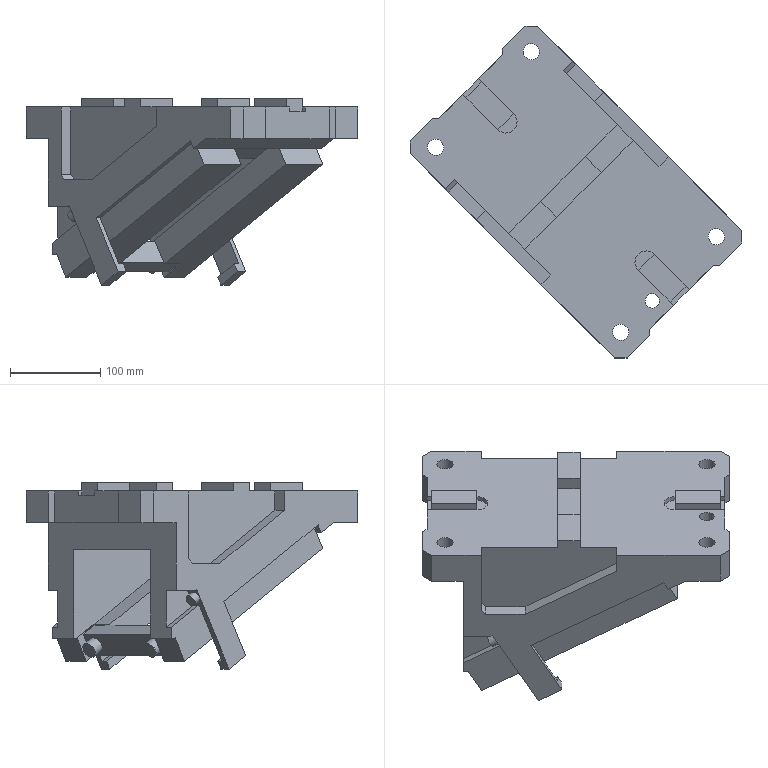Part | NX | features solid 2 | 1 solid | 151 faces | box 367.696 x 367.696 x 206.368 mm | volume 4417442 mm3 | plane 131 | cylinder 18 | cone 2 | commonest cylinder face diameters 18 x6 26 x4 13 x2 16 x2 25 x2 32 x2